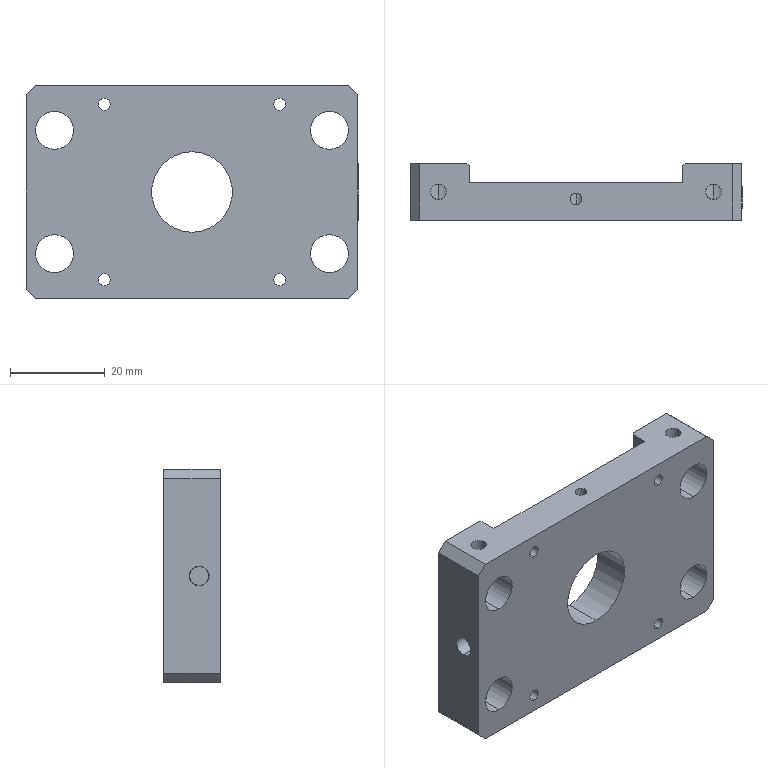Part | SolidWorks | features ICE 8, HoleWzd 6, 3DProfileFeature 4, Chamfer 2, CirPattern 1, Extrusion 1, MirrorPattern 1 | 1 solid | 70 faces | box 70 x 12 x 45 mm | volume 24347 mm3 | cylinder 46 | plane 20 | cone 4 | commonest cylinder face diameters 2.5 x16 3 x8 3.3 x8 8 x8 4 x2 4.2 x2